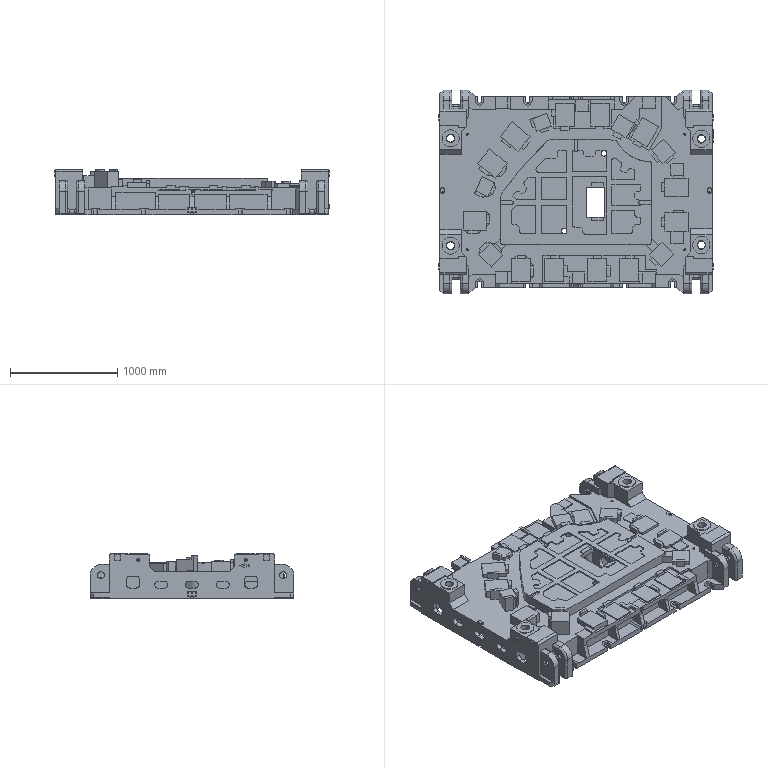Part | NX | features solid 2 | 1 solid | 1720 faces | box 2560 x 1900 x 425 mm | volume 538571806 mm3 | plane 1399 | cylinder 271 | spline 34 | torus 16 | commonest cylinder face diameters 60 x82 68 x48 40 x32 50 x20 30 x16 64 x16